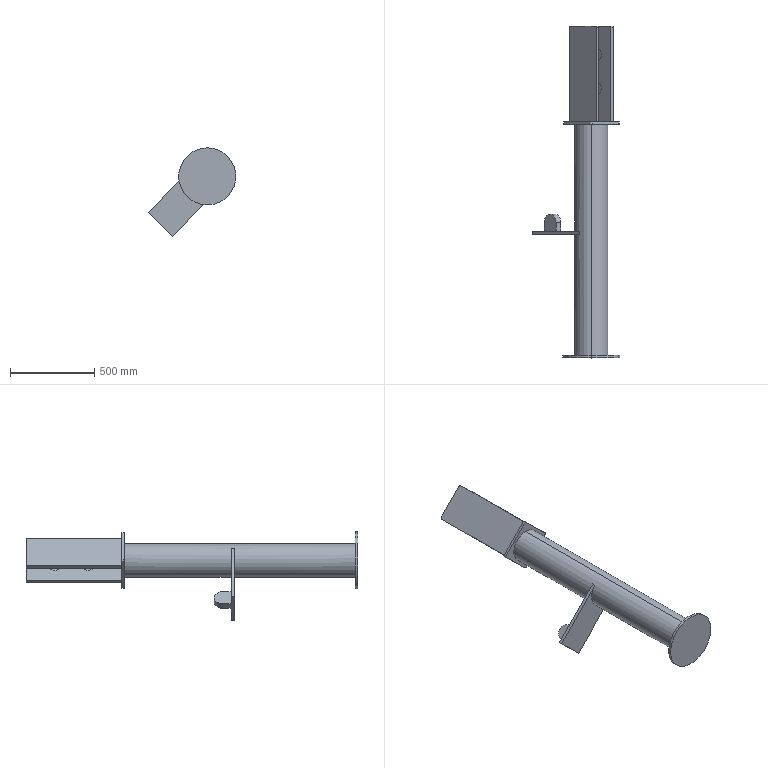Part | SolidWorks | features BaseBody 1 | 1 solid | 53 faces | box 521.246 x 1975 x 525.819 mm | volume 52229726 mm3 | plane 31 | cylinder 22 | commonest cylinder face diameters 20 x9 70 x8 200 x2 340 x2 100 x1